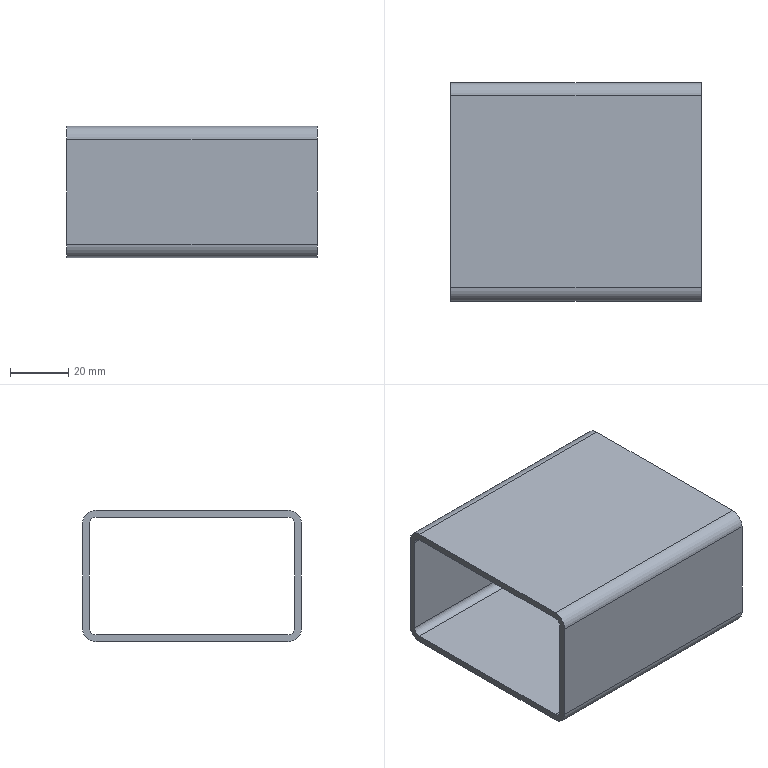Part | STEP file | [03]-8 | 1 solid | 18 faces | box 86.001 x 75 x 45 mm | volume 44481 mm3 | plane 10 | cylinder 8 | commonest cylinder face diameters 4.6 x4 9.2 x4
STEP:
#1=CARTESIAN_POINT('',(86.001,70.4,45.));
#2=VERTEX_POINT('',#1);
#3=CARTESIAN_POINT('',(86.001,4.6,45.));
#4=VERTEX_POINT('',#3);
#5=CARTESIAN_POINT('',(86.001,70.4,45.));
#6=DIRECTION('',(0.,-1.,0.));
#7=VECTOR('',#6,1000.);
#8=LINE('',#5,#7);
#9=EDGE_CURVE('',#2,#4,#8,.T.);
#10=ORIENTED_EDGE('',*,*,#9,.T.);
#11=CARTESIAN_POINT('',(86.001,0.,40.4));
#12=VERTEX_POINT('',#11);
#13=CARTESIAN_POINT('',(86.001,4.6,40.4));
#14=DIRECTION('',(1.,0.,0.));
#15=DIRECTION('',(0.,0.,1.));
#16=AXIS2_PLACEMENT_3D('',#13,#14,#15);
#17=CIRCLE('',#16,4.6);
#18=EDGE_CURVE('',#4,#12,#17,.T.);
#19=ORIENTED_EDGE('',*,*,#18,.T.);
#20=CARTESIAN_POINT('',(86.001,0.,4.6));
#21=VERTEX_POINT('',#20);
#22=CARTESIAN_POINT('',(86.001,0.,40.4));
#23=DIRECTION('',(0.,0.,-1.));
#24=VECTOR('',#23,1000.);
#25=LINE('',#22,#24);
#26=EDGE_CURVE('',#12,#21,#25,.T.);
#27=ORIENTED_EDGE('',*,*,#26,.T.);
#28=CARTESIAN_POINT('',(86.001,4.6,0.));
#29=VERTEX_POINT('',#28);
#30=CARTESIAN_POINT('',(86.001,4.6,4.6));
#31=DIRECTION('',(1.,0.,0.));
#32=DIRECTION('',(0.,0.,1.));
#33=AXIS2_PLACEMENT_3D('',#30,#31,#32);
#34=CIRCLE('',#33,4.6);
#35=EDGE_CURVE('',#21,#29,#34,.T.);
#36=ORIENTED_EDGE('',*,*,#35,.T.);
#37=CARTESIAN_POINT('',(86.001,70.4,0.));
#38=VERTEX_POINT('',#37);
#39=CARTESIAN_POINT('',(86.001,4.6,0.));
#40=DIRECTION('',(0.,1.,0.));
#41=VECTOR('',#40,1000.);
#42=LINE('',#39,#41);
#43=EDGE_CURVE('',#29,#38,#42,.T.);
#44=ORIENTED_EDGE('',*,*,#43,.T.);
#45=CARTESIAN_POINT('',(86.001,75.,4.6));
#46=VERTEX_POINT('',#45);
#47=CARTESIAN_POINT('',(86.001,70.4,4.6));
#48=DIRECTION('',(1.,0.,0.));
#49=DIRECTION('',(0.,0.,1.));
#50=AXIS2_PLACEMENT_3D('',#47,#48,#49);
#51=CIRCLE('',#50,4.6);
#52=EDGE_CURVE('',#38,#46,#51,.T.);
#53=ORIENTED_EDGE('',*,*,#52,.T.);
#54=CARTESIAN_POINT('',(86.001,75.,40.4));
#55=VERTEX_POINT('',#54);
#56=CARTESIAN_POINT('',(86.001,75.,4.6));
#57=DIRECTION('',(0.,0.,1.));
#58=VECTOR('',#57,1000.);
#59=LINE('',#56,#58);
#60=EDGE_CURVE('',#46,#55,#59,.T.);
#61=ORIENTED_EDGE('',*,*,#60,.T.);
#62=CARTESIAN_POINT('',(86.001,70.4,40.4));
#63=DIRECTION('',(1.,0.,0.));
#64=DIRECTION('',(0.,0.,1.));
#65=AXIS2_PLACEMENT_3D('',#62,#63,#64);
#66=CIRCLE('',#65,4.6);
#67=EDGE_CURVE('',#55,#2,#66,.T.);
#68=ORIENTED_EDGE('',*,*,#67,.T.);
#69=EDGE_LOOP('',(#10,#19,#27,#36,#44,#53,#61,#68));
#70=FACE_OUTER_BOUND('',#69,.T.);
#71=CARTESIAN_POINT('',(86.001,70.4,42.7));
#72=VERTEX_POINT('',#71);
#73=CARTESIAN_POINT('',(86.001,4.6,42.7));
#74=VERTEX_POINT('',#73);
#75=CARTESIAN_POINT('',(86.001,70.4,42.7));
#76=DIRECTION('',(0.,-1.,0.));
#77=VECTOR('',#76,1000.);
#78=LINE('',#75,#77);
#79=EDGE_CURVE('',#72,#74,#78,.T.);
#80=ORIENTED_EDGE('',*,*,#79,.F.);
#81=CARTESIAN_POINT('',(86.001,72.7,40.4));
#82=VERTEX_POINT('',#81);
#83=CARTESIAN_POINT('',(86.001,70.4,40.4));
#84=DIRECTION('',(1.,0.,0.));
#85=DIRECTION('',(0.,1.,0.));
#86=AXIS2_PLACEMENT_3D('',#83,#84,#85);
#87=CIRCLE('',#86,2.3);
#88=EDGE_CURVE('',#82,#72,#87,.T.);
#89=ORIENTED_EDGE('',*,*,#88,.F.);
#90=CARTESIAN_POINT('',(86.001,72.7,4.6));
#91=VERTEX_POINT('',#90);
#92=CARTESIAN_POINT('',(86.001,72.7,4.6));
#93=DIRECTION('',(0.,0.,1.));
#94=VECTOR('',#93,1000.);
#95=LINE('',#92,#94);
#96=EDGE_CURVE('',#91,#82,#95,.T.);
#97=ORIENTED_EDGE('',*,*,#96,.F.);
#98=CARTESIAN_POINT('',(86.001,70.4,2.3));
#99=VERTEX_POINT('',#98);
#100=CARTESIAN_POINT('',(86.001,70.4,4.6));
#101=DIRECTION('',(1.,0.,0.));
#102=DIRECTION('',(0.,1.,0.));
#103=AXIS2_PLACEMENT_3D('',#100,#101,#102);
#104=CIRCLE('',#103,2.3);
#105=EDGE_CURVE('',#99,#91,#104,.T.);
#106=ORIENTED_EDGE('',*,*,#105,.F.);
#107=CARTESIAN_POINT('',(86.001,4.6,2.3));
#108=VERTEX_POINT('',#107);
#109=CARTESIAN_POINT('',(86.001,4.6,2.3));
#110=DIRECTION('',(0.,1.,0.));
#111=VECTOR('',#110,1000.);
#112=LINE('',#109,#111);
#113=EDGE_CURVE('',#108,#99,#112,.T.);
#114=ORIENTED_EDGE('',*,*,#113,.F.);
#115=CARTESIAN_POINT('',(86.001,2.3,4.6));
#116=VERTEX_POINT('',#115);
#117=CARTESIAN_POINT('',(86.001,4.6,4.6));
#118=DIRECTION('',(1.,0.,0.));
#119=DIRECTION('',(0.,1.,0.));
#120=AXIS2_PLACEMENT_3D('',#117,#118,#119);
#121=CIRCLE('',#120,2.3);
#122=EDGE_CURVE('',#116,#108,#121,.T.);
#123=ORIENTED_EDGE('',*,*,#122,.F.);
#124=CARTESIAN_POINT('',(86.001,2.3,40.4));
#125=VERTEX_POINT('',#124);
#126=CARTESIAN_POINT('',(86.001,2.3,40.4));
#127=DIRECTION('',(0.,0.,-1.));
#128=VECTOR('',#127,1000.);
#129=LINE('',#126,#128);
#130=EDGE_CURVE('',#125,#116,#129,.T.);
#131=ORIENTED_EDGE('',*,*,#130,.F.);
#132=CARTESIAN_POINT('',(86.001,4.6,40.4));
#133=DIRECTION('',(1.,0.,0.));
#134=DIRECTION('',(0.,1.,0.));
#135=AXIS2_PLACEMENT_3D('',#132,#133,#134);
#136=CIRCLE('',#135,2.3);
#137=EDGE_CURVE('',#74,#125,#136,.T.);
#138=ORIENTED_EDGE('',*,*,#137,.F.);
#139=EDGE_LOOP('',(#80,#89,#97,#106,#114,#123,#131,#138));
#140=FACE_BOUND('',#139,.T.);
#141=CARTESIAN_POINT('',(86.001,4.6,40.4));
#142=DIRECTION('',(1.,0.,0.));
#143=DIRECTION('',(0.,0.,1.));
#144=AXIS2_PLACEMENT_3D('',#141,#142,#143);
#145=PLANE('',#144);
#146=ADVANCED_FACE('',(#70,#140),#145,.T.);
#147=CARTESIAN_POINT('',(0.,70.4,45.));
#148=VERTEX_POINT('',#147);
#149=CARTESIAN_POINT('',(0.,4.6,45.));
#150=VERTEX_POINT('',#149);
#151=CARTESIAN_POINT('',(0.,70.4,45.));
#152=DIRECTION('',(0.,-1.,0.));
#153=VECTOR('',#152,1000.);
#154=LINE('',#151,#153);
#155=EDGE_CURVE('',#148,#150,#154,.T.);
#156=ORIENTED_EDGE('',*,*,#155,.F.);
#157=CARTESIAN_POINT('',(0.,75.,40.4));
#158=VERTEX_POINT('',#157);
#159=CARTESIAN_POINT('',(0.,70.4,40.4));
#160=DIRECTION('',(1.,0.,0.));
#161=DIRECTION('',(0.,0.,1.));
#162=AXIS2_PLACEMENT_3D('',#159,#160,#161);
#163=CIRCLE('',#162,4.6);
#164=EDGE_CURVE('',#158,#148,#163,.T.);
#165=ORIENTED_EDGE('',*,*,#164,.F.);
#166=CARTESIAN_POINT('',(0.,75.,4.6));
#167=VERTEX_POINT('',#166);
#168=CARTESIAN_POINT('',(0.,75.,4.6));
#169=DIRECTION('',(0.,0.,1.));
#170=VECTOR('',#169,1000.);
#171=LINE('',#168,#170);
#172=EDGE_CURVE('',#167,#158,#171,.T.);
#173=ORIENTED_EDGE('',*,*,#172,.F.);
#174=CARTESIAN_POINT('',(0.,70.4,0.));
#175=VERTEX_POINT('',#174);
#176=CARTESIAN_POINT('',(0.,70.4,4.6));
#177=DIRECTION('',(1.,0.,0.));
#178=DIRECTION('',(0.,0.,1.));
#179=AXIS2_PLACEMENT_3D('',#176,#177,#178);
#180=CIRCLE('',#179,4.6);
#181=EDGE_CURVE('',#175,#167,#180,.T.);
#182=ORIENTED_EDGE('',*,*,#181,.F.);
#183=CARTESIAN_POINT('',(0.,4.6,0.));
#184=VERTEX_POINT('',#183);
#185=CARTESIAN_POINT('',(0.,4.6,0.));
#186=DIRECTION('',(0.,1.,0.));
#187=VECTOR('',#186,1000.);
#188=LINE('',#185,#187);
#189=EDGE_CURVE('',#184,#175,#188,.T.);
#190=ORIENTED_EDGE('',*,*,#189,.F.);
#191=CARTESIAN_POINT('',(0.,0.,4.6));
#192=VERTEX_POINT('',#191);
#193=CARTESIAN_POINT('',(0.,4.6,4.6));
#194=DIRECTION('',(1.,0.,0.));
#195=DIRECTION('',(0.,0.,1.));
#196=AXIS2_PLACEMENT_3D('',#193,#194,#195);
#197=CIRCLE('',#196,4.6);
#198=EDGE_CURVE('',#192,#184,#197,.T.);
#199=ORIENTED_EDGE('',*,*,#198,.F.);
#200=CARTESIAN_POINT('',(0.,0.,40.4));
#201=VERTEX_POINT('',#200);
#202=CARTESIAN_POINT('',(0.,0.,40.4));
#203=DIRECTION('',(0.,0.,-1.));
#204=VECTOR('',#203,1000.);
#205=LINE('',#202,#204);
#206=EDGE_CURVE('',#201,#192,#205,.T.);
#207=ORIENTED_EDGE('',*,*,#206,.F.);
#208=CARTESIAN_POINT('',(0.,4.6,40.4));
#209=DIRECTION('',(1.,0.,0.));
#210=DIRECTION('',(0.,0.,1.));
#211=AXIS2_PLACEMENT_3D('',#208,#209,#210);
#212=CIRCLE('',#211,4.6);
#213=EDGE_CURVE('',#150,#201,#212,.T.);
#214=ORIENTED_EDGE('',*,*,#213,.F.);
#215=EDGE_LOOP('',(#156,#165,#173,#182,#190,#199,#207,#214));
#216=FACE_OUTER_BOUND('',#215,.T.);
#217=CARTESIAN_POINT('',(0.,72.7,40.4));
#218=VERTEX_POINT('',#217);
#219=CARTESIAN_POINT('',(0.,70.4,42.7));
#220=VERTEX_POINT('',#219);
#221=CARTESIAN_POINT('',(0.,70.4,40.4));
#222=DIRECTION('',(1.,0.,0.));
#223=DIRECTION('',(0.,1.,0.));
#224=AXIS2_PLACEMENT_3D('',#221,#222,#223);
#225=CIRCLE('',#224,2.3);
#226=EDGE_CURVE('',#218,#220,#225,.T.);
#227=ORIENTED_EDGE('',*,*,#226,.T.);
#228=CARTESIAN_POINT('',(0.,4.6,42.7));
#229=VERTEX_POINT('',#228);
#230=CARTESIAN_POINT('',(0.,70.4,42.7));
#231=DIRECTION('',(0.,-1.,0.));
#232=VECTOR('',#231,1000.);
#233=LINE('',#230,#232);
#234=EDGE_CURVE('',#220,#229,#233,.T.);
#235=ORIENTED_EDGE('',*,*,#234,.T.);
#236=CARTESIAN_POINT('',(0.,2.3,40.4));
#237=VERTEX_POINT('',#236);
#238=CARTESIAN_POINT('',(0.,4.6,40.4));
#239=DIRECTION('',(1.,0.,0.));
#240=DIRECTION('',(0.,1.,0.));
#241=AXIS2_PLACEMENT_3D('',#238,#239,#240);
#242=CIRCLE('',#241,2.3);
#243=EDGE_CURVE('',#229,#237,#242,.T.);
#244=ORIENTED_EDGE('',*,*,#243,.T.);
#245=CARTESIAN_POINT('',(0.,2.3,4.6));
#246=VERTEX_POINT('',#245);
#247=CARTESIAN_POINT('',(0.,2.3,40.4));
#248=DIRECTION('',(0.,0.,-1.));
#249=VECTOR('',#248,1000.);
#250=LINE('',#247,#249);
#251=EDGE_CURVE('',#237,#246,#250,.T.);
#252=ORIENTED_EDGE('',*,*,#251,.T.);
#253=CARTESIAN_POINT('',(0.,4.6,2.3));
#254=VERTEX_POINT('',#253);
#255=CARTESIAN_POINT('',(0.,4.6,4.6));
#256=DIRECTION('',(1.,0.,0.));
#257=DIRECTION('',(0.,1.,0.));
#258=AXIS2_PLACEMENT_3D('',#255,#256,#257);
#259=CIRCLE('',#258,2.3);
#260=EDGE_CURVE('',#246,#254,#259,.T.);
#261=ORIENTED_EDGE('',*,*,#260,.T.);
#262=CARTESIAN_POINT('',(0.,70.4,2.3));
#263=VERTEX_POINT('',#262);
#264=CARTESIAN_POINT('',(0.,4.6,2.3));
#265=DIRECTION('',(0.,1.,0.));
#266=VECTOR('',#265,1000.);
#267=LINE('',#264,#266);
#268=EDGE_CURVE('',#254,#263,#267,.T.);
#269=ORIENTED_EDGE('',*,*,#268,.T.);
#270=CARTESIAN_POINT('',(0.,72.7,4.6));
#271=VERTEX_POINT('',#270);
#272=CARTESIAN_POINT('',(0.,70.4,4.6));
#273=DIRECTION('',(1.,0.,0.));
#274=DIRECTION('',(0.,1.,0.));
#275=AXIS2_PLACEMENT_3D('',#272,#273,#274);
#276=CIRCLE('',#275,2.3);
#277=EDGE_CURVE('',#263,#271,#276,.T.);
#278=ORIENTED_EDGE('',*,*,#277,.T.);
#279=CARTESIAN_POINT('',(0.,72.7,4.6));
#280=DIRECTION('',(0.,0.,1.));
#281=VECTOR('',#280,1000.);
#282=LINE('',#279,#281);
#283=EDGE_CURVE('',#271,#218,#282,.T.);
#284=ORIENTED_EDGE('',*,*,#283,.T.);
#285=EDGE_LOOP('',(#227,#235,#244,#252,#261,#269,#278,#284));
#286=FACE_BOUND('',#285,.T.);
#287=CARTESIAN_POINT('',(0.,4.6,40.4));
#288=DIRECTION('',(1.,0.,0.));
#289=DIRECTION('',(0.,0.,1.));
#290=AXIS2_PLACEMENT_3D('',#287,#288,#289);
#291=PLANE('',#290);
#292=ADVANCED_FACE('',(#216,#286),#291,.F.);
#293=ORIENTED_EDGE('',*,*,#155,.T.);
#294=CARTESIAN_POINT('',(86.001,4.6,45.));
#295=DIRECTION('',(-1.,0.,0.));
#296=VECTOR('',#295,1000.);
#297=LINE('',#294,#296);
#298=EDGE_CURVE('',#4,#150,#297,.T.);
#299=ORIENTED_EDGE('',*,*,#298,.F.);
#300=ORIENTED_EDGE('',*,*,#9,.F.);
#301=CARTESIAN_POINT('',(86.001,70.4,45.));
#302=DIRECTION('',(-1.,0.,0.));
#303=VECTOR('',#302,1000.);
#304=LINE('',#301,#303);
#305=EDGE_CURVE('',#2,#148,#304,.T.);
#306=ORIENTED_EDGE('',*,*,#305,.T.);
#307=EDGE_LOOP('',(#293,#299,#300,#306));
#308=FACE_OUTER_BOUND('',#307,.T.);
#309=CARTESIAN_POINT('',(86.001,70.4,45.));
#310=DIRECTION('',(0.,0.,-1.));
#311=DIRECTION('',(0.,1.,0.));
#312=AXIS2_PLACEMENT_3D('',#309,#310,#311);
#313=PLANE('',#312);
#314=ADVANCED_FACE('',(#308),#313,.F.);
#315=ORIENTED_EDGE('',*,*,#213,.T.);
#316=CARTESIAN_POINT('',(86.001,0.,40.4));
#317=DIRECTION('',(-1.,0.,0.));
#318=VECTOR('',#317,1000.);
#319=LINE('',#316,#318);
#320=EDGE_CURVE('',#12,#201,#319,.T.);
#321=ORIENTED_EDGE('',*,*,#320,.F.);
#322=ORIENTED_EDGE('',*,*,#18,.F.);
#323=ORIENTED_EDGE('',*,*,#298,.T.);
#324=EDGE_LOOP('',(#315,#321,#322,#323));
#325=FACE_OUTER_BOUND('',#324,.T.);
#326=CARTESIAN_POINT('',(86.001,4.6,40.4));
#327=DIRECTION('',(-1.,0.,0.));
#328=DIRECTION('',(0.,0.,-1.));
#329=AXIS2_PLACEMENT_3D('',#326,#327,#328);
#330=CYLINDRICAL_SURFACE('',#329,4.6);
#331=ADVANCED_FACE('',(#325),#330,.T.);
#332=ORIENTED_EDGE('',*,*,#206,.T.);
#333=CARTESIAN_POINT('',(86.001,0.,4.6));
#334=DIRECTION('',(-1.,0.,0.));
#335=VECTOR('',#334,1000.);
#336=LINE('',#333,#335);
#337=EDGE_CURVE('',#21,#192,#336,.T.);
#338=ORIENTED_EDGE('',*,*,#337,.F.);
#339=ORIENTED_EDGE('',*,*,#26,.F.);
#340=ORIENTED_EDGE('',*,*,#320,.T.);
#341=EDGE_LOOP('',(#332,#338,#339,#340));
#342=FACE_OUTER_BOUND('',#341,.T.);
#343=CARTESIAN_POINT('',(86.001,0.,40.4));
#344=DIRECTION('',(0.,1.,0.));
#345=DIRECTION('',(0.,0.,1.));
#346=AXIS2_PLACEMENT_3D('',#343,#344,#345);
#347=PLANE('',#346);
#348=ADVANCED_FACE('',(#342),#347,.F.);
#349=ORIENTED_EDGE('',*,*,#198,.T.);
#350=CARTESIAN_POINT('',(86.001,4.6,0.));
#351=DIRECTION('',(-1.,0.,0.));
#352=VECTOR('',#351,1000.);
#353=LINE('',#350,#352);
#354=EDGE_CURVE('',#29,#184,#353,.T.);
#355=ORIENTED_EDGE('',*,*,#354,.F.);
#356=ORIENTED_EDGE('',*,*,#35,.F.);
#357=ORIENTED_EDGE('',*,*,#337,.T.);
#358=EDGE_LOOP('',(#349,#355,#356,#357));
#359=FACE_OUTER_BOUND('',#358,.T.);
#360=CARTESIAN_POINT('',(86.001,4.6,4.6));
#361=DIRECTION('',(-1.,0.,0.));
#362=DIRECTION('',(0.,0.,-1.));
#363=AXIS2_PLACEMENT_3D('',#360,#361,#362);
#364=CYLINDRICAL_SURFACE('',#363,4.6);
#365=ADVANCED_FACE('',(#359),#364,.T.);
#366=ORIENTED_EDGE('',*,*,#189,.T.);
#367=CARTESIAN_POINT('',(86.001,70.4,0.));
#368=DIRECTION('',(-1.,0.,0.));
#369=VECTOR('',#368,1000.);
#370=LINE('',#367,#369);
#371=EDGE_CURVE('',#38,#175,#370,.T.);
#372=ORIENTED_EDGE('',*,*,#371,.F.);
#373=ORIENTED_EDGE('',*,*,#43,.F.);
#374=ORIENTED_EDGE('',*,*,#354,.T.);
#375=EDGE_LOOP('',(#366,#372,#373,#374));
#376=FACE_OUTER_BOUND('',#375,.T.);
#377=CARTESIAN_POINT('',(86.001,4.6,0.));
#378=DIRECTION('',(0.,0.,1.));
#379=DIRECTION('',(0.,-1.,0.));
#380=AXIS2_PLACEMENT_3D('',#377,#378,#379);
#381=PLANE('',#380);
#382=ADVANCED_FACE('',(#376),#381,.F.);
#383=ORIENTED_EDGE('',*,*,#181,.T.);
#384=CARTESIAN_POINT('',(86.001,75.,4.6));
#385=DIRECTION('',(-1.,0.,0.));
#386=VECTOR('',#385,1000.);
#387=LINE('',#384,#386);
#388=EDGE_CURVE('',#46,#167,#387,.T.);
#389=ORIENTED_EDGE('',*,*,#388,.F.);
#390=ORIENTED_EDGE('',*,*,#52,.F.);
#391=ORIENTED_EDGE('',*,*,#371,.T.);
#392=EDGE_LOOP('',(#383,#389,#390,#391));
#393=FACE_OUTER_BOUND('',#392,.T.);
#394=CARTESIAN_POINT('',(86.001,70.4,4.6));
#395=DIRECTION('',(-1.,0.,0.));
#396=DIRECTION('',(0.,0.,-1.));
#397=AXIS2_PLACEMENT_3D('',#394,#395,#396);
#398=CYLINDRICAL_SURFACE('',#397,4.6);
#399=ADVANCED_FACE('',(#393),#398,.T.);
#400=ORIENTED_EDGE('',*,*,#172,.T.);
#401=CARTESIAN_POINT('',(86.001,75.,40.4));
#402=DIRECTION('',(-1.,0.,0.));
#403=VECTOR('',#402,1000.);
#404=LINE('',#401,#403);
#405=EDGE_CURVE('',#55,#158,#404,.T.);
#406=ORIENTED_EDGE('',*,*,#405,.F.);
#407=ORIENTED_EDGE('',*,*,#60,.F.);
#408=ORIENTED_EDGE('',*,*,#388,.T.);
#409=EDGE_LOOP('',(#400,#406,#407,#408));
#410=FACE_OUTER_BOUND('',#409,.T.);
#411=CARTESIAN_POINT('',(86.001,75.,4.6));
#412=DIRECTION('',(0.,-1.,0.));
#413=DIRECTION('',(1.,0.,0.));
#414=AXIS2_PLACEMENT_3D('',#411,#412,#413);
#415=PLANE('',#414);
#416=ADVANCED_FACE('',(#410),#415,.F.);
#417=ORIENTED_EDGE('',*,*,#164,.T.);
#418=ORIENTED_EDGE('',*,*,#305,.F.);
#419=ORIENTED_EDGE('',*,*,#67,.F.);
#420=ORIENTED_EDGE('',*,*,#405,.T.);
#421=EDGE_LOOP('',(#417,#418,#419,#420));
#422=FACE_OUTER_BOUND('',#421,.T.);
#423=CARTESIAN_POINT('',(86.001,70.4,40.4));
#424=DIRECTION('',(-1.,0.,0.));
#425=DIRECTION('',(0.,0.,-1.));
#426=AXIS2_PLACEMENT_3D('',#423,#424,#425);
#427=CYLINDRICAL_SURFACE('',#426,4.6);
#428=ADVANCED_FACE('',(#422),#427,.T.);
#429=ORIENTED_EDGE('',*,*,#226,.F.);
#430=CARTESIAN_POINT('',(86.001,72.7,40.4));
#431=DIRECTION('',(-1.,0.,0.));
#432=VECTOR('',#431,1000.);
#433=LINE('',#430,#432);
#434=EDGE_CURVE('',#82,#218,#433,.T.);
#435=ORIENTED_EDGE('',*,*,#434,.F.);
#436=ORIENTED_EDGE('',*,*,#88,.T.);
#437=CARTESIAN_POINT('',(86.001,70.4,42.7));
#438=DIRECTION('',(-1.,0.,0.));
#439=VECTOR('',#438,1000.);
#440=LINE('',#437,#439);
#441=EDGE_CURVE('',#72,#220,#440,.T.);
#442=ORIENTED_EDGE('',*,*,#441,.T.);
#443=EDGE_LOOP('',(#429,#435,#436,#442));
#444=FACE_OUTER_BOUND('',#443,.T.);
#445=CARTESIAN_POINT('',(86.001,70.4,40.4));
#446=DIRECTION('',(-1.,0.,0.));
#447=DIRECTION('',(0.,-1.,0.));
#448=AXIS2_PLACEMENT_3D('',#445,#446,#447);
#449=CYLINDRICAL_SURFACE('',#448,2.3);
#450=ADVANCED_FACE('',(#444),#449,.F.);
#451=ORIENTED_EDGE('',*,*,#234,.F.);
#452=ORIENTED_EDGE('',*,*,#441,.F.);
#453=ORIENTED_EDGE('',*,*,#79,.T.);
#454=CARTESIAN_POINT('',(86.001,4.6,42.7));
#455=DIRECTION('',(-1.,0.,0.));
#456=VECTOR('',#455,1000.);
#457=LINE('',#454,#456);
#458=EDGE_CURVE('',#74,#229,#457,.T.);
#459=ORIENTED_EDGE('',*,*,#458,.T.);
#460=EDGE_LOOP('',(#451,#452,#453,#459));
#461=FACE_OUTER_BOUND('',#460,.T.);
#462=CARTESIAN_POINT('',(86.001,70.4,42.7));
#463=DIRECTION('',(0.,0.,-1.));
#464=DIRECTION('',(-1.,0.,0.));
#465=AXIS2_PLACEMENT_3D('',#462,#463,#464);
#466=PLANE('',#465);
#467=ADVANCED_FACE('',(#461),#466,.T.);
#468=ORIENTED_EDGE('',*,*,#243,.F.);
#469=ORIENTED_EDGE('',*,*,#458,.F.);
#470=ORIENTED_EDGE('',*,*,#137,.T.);
#471=CARTESIAN_POINT('',(86.001,2.3,40.4));
#472=DIRECTION('',(-1.,0.,0.));
#473=VECTOR('',#472,1000.);
#474=LINE('',#471,#473);
#475=EDGE_CURVE('',#125,#237,#474,.T.);
#476=ORIENTED_EDGE('',*,*,#475,.T.);
#477=EDGE_LOOP('',(#468,#469,#470,#476));
#478=FACE_OUTER_BOUND('',#477,.T.);
#479=CARTESIAN_POINT('',(86.001,4.6,40.4));
#480=DIRECTION('',(-1.,0.,0.));
#481=DIRECTION('',(0.,-1.,0.));
#482=AXIS2_PLACEMENT_3D('',#479,#480,#481);
#483=CYLINDRICAL_SURFACE('',#482,2.3);
#484=ADVANCED_FACE('',(#478),#483,.F.);
#485=ORIENTED_EDGE('',*,*,#251,.F.);
#486=ORIENTED_EDGE('',*,*,#475,.F.);
#487=ORIENTED_EDGE('',*,*,#130,.T.);
#488=CARTESIAN_POINT('',(86.001,2.3,4.6));
#489=DIRECTION('',(-1.,0.,0.));
#490=VECTOR('',#489,1000.);
#491=LINE('',#488,#490);
#492=EDGE_CURVE('',#116,#246,#491,.T.);
#493=ORIENTED_EDGE('',*,*,#492,.T.);
#494=EDGE_LOOP('',(#485,#486,#487,#493));
#495=FACE_OUTER_BOUND('',#494,.T.);
#496=CARTESIAN_POINT('',(86.001,2.3,40.4));
#497=DIRECTION('',(0.,1.,0.));
#498=DIRECTION('',(-1.,0.,0.));
#499=AXIS2_PLACEMENT_3D('',#496,#497,#498);
#500=PLANE('',#499);
#501=ADVANCED_FACE('',(#495),#500,.T.);
#502=ORIENTED_EDGE('',*,*,#260,.F.);
#503=ORIENTED_EDGE('',*,*,#492,.F.);
#504=ORIENTED_EDGE('',*,*,#122,.T.);
#505=CARTESIAN_POINT('',(86.001,4.6,2.3));
#506=DIRECTION('',(-1.,0.,0.));
#507=VECTOR('',#506,1000.);
#508=LINE('',#505,#507);
#509=EDGE_CURVE('',#108,#254,#508,.T.);
#510=ORIENTED_EDGE('',*,*,#509,.T.);
#511=EDGE_LOOP('',(#502,#503,#504,#510));
#512=FACE_OUTER_BOUND('',#511,.T.);
#513=CARTESIAN_POINT('',(86.001,4.6,4.6));
#514=DIRECTION('',(-1.,0.,0.));
#515=DIRECTION('',(0.,-1.,0.));
#516=AXIS2_PLACEMENT_3D('',#513,#514,#515);
#517=CYLINDRICAL_SURFACE('',#516,2.3);
#518=ADVANCED_FACE('',(#512),#517,.F.);
#519=ORIENTED_EDGE('',*,*,#268,.F.);
#520=ORIENTED_EDGE('',*,*,#509,.F.);
#521=ORIENTED_EDGE('',*,*,#113,.T.);
#522=CARTESIAN_POINT('',(86.001,70.4,2.3));
#523=DIRECTION('',(-1.,0.,0.));
#524=VECTOR('',#523,1000.);
#525=LINE('',#522,#524);
#526=EDGE_CURVE('',#99,#263,#525,.T.);
#527=ORIENTED_EDGE('',*,*,#526,.T.);
#528=EDGE_LOOP('',(#519,#520,#521,#527));
#529=FACE_OUTER_BOUND('',#528,.T.);
#530=CARTESIAN_POINT('',(86.001,4.6,2.3));
#531=DIRECTION('',(0.,0.,1.));
#532=DIRECTION('',(0.,-1.,0.));
#533=AXIS2_PLACEMENT_3D('',#530,#531,#532);
#534=PLANE('',#533);
#535=ADVANCED_FACE('',(#529),#534,.T.);
#536=ORIENTED_EDGE('',*,*,#277,.F.);
#537=ORIENTED_EDGE('',*,*,#526,.F.);
#538=ORIENTED_EDGE('',*,*,#105,.T.);
#539=CARTESIAN_POINT('',(86.001,72.7,4.6));
#540=DIRECTION('',(-1.,0.,0.));
#541=VECTOR('',#540,1000.);
#542=LINE('',#539,#541);
#543=EDGE_CURVE('',#91,#271,#542,.T.);
#544=ORIENTED_EDGE('',*,*,#543,.T.);
#545=EDGE_LOOP('',(#536,#537,#538,#544));
#546=FACE_OUTER_BOUND('',#545,.T.);
#547=CARTESIAN_POINT('',(86.001,70.4,4.6));
#548=DIRECTION('',(-1.,0.,0.));
#549=DIRECTION('',(0.,-1.,0.));
#550=AXIS2_PLACEMENT_3D('',#547,#548,#549);
#551=CYLINDRICAL_SURFACE('',#550,2.3);
#552=ADVANCED_FACE('',(#546),#551,.F.);
#553=ORIENTED_EDGE('',*,*,#283,.F.);
#554=ORIENTED_EDGE('',*,*,#543,.F.);
#555=ORIENTED_EDGE('',*,*,#96,.T.);
#556=ORIENTED_EDGE('',*,*,#434,.T.);
#557=EDGE_LOOP('',(#553,#554,#555,#556));
#558=FACE_OUTER_BOUND('',#557,.T.);
#559=CARTESIAN_POINT('',(86.001,72.7,4.6));
#560=DIRECTION('',(0.,-1.,0.));
#561=DIRECTION('',(0.,0.,-1.));
#562=AXIS2_PLACEMENT_3D('',#559,#560,#561);
#563=PLANE('',#562);
#564=ADVANCED_FACE('',(#558),#563,.T.);
#565=CLOSED_SHELL('',(#146,#292,#314,#331,#348,#365,#382,#399,#416,#428,#450,#467,#484,#501,#518,#535,#552,#564));
#566=MANIFOLD_SOLID_BREP('',#565);
#567=CARTESIAN_POINT('',(0.,0.,0.));
#568=DIRECTION('',(0.,0.,1.));
#569=DIRECTION('',(1.,0.,0.));
#570=AXIS2_PLACEMENT_3D('',#567,#568,#569);
#571=(LENGTH_UNIT()NAMED_UNIT(*)SI_UNIT(.MILLI.,.METRE.));
#572=UNCERTAINTY_MEASURE_WITH_UNIT(LENGTH_MEASURE(0.00001),#571,'','');
#573=(NAMED_UNIT(*)PLANE_ANGLE_UNIT()SI_UNIT($,.RADIAN.));
#574=(NAMED_UNIT(*)SI_UNIT($,.STERADIAN.)SOLID_ANGLE_UNIT());
#575=(GEOMETRIC_REPRESENTATION_CONTEXT(3)GLOBAL_UNCERTAINTY_ASSIGNED_CONTEXT((#572))GLOBAL_UNIT_ASSIGNED_CONTEXT((#571,#573,#574))REPRESENTATION_CONTEXT('',''));
#576=ADVANCED_BREP_SHAPE_REPRESENTATION('',(#566,#570),#575);